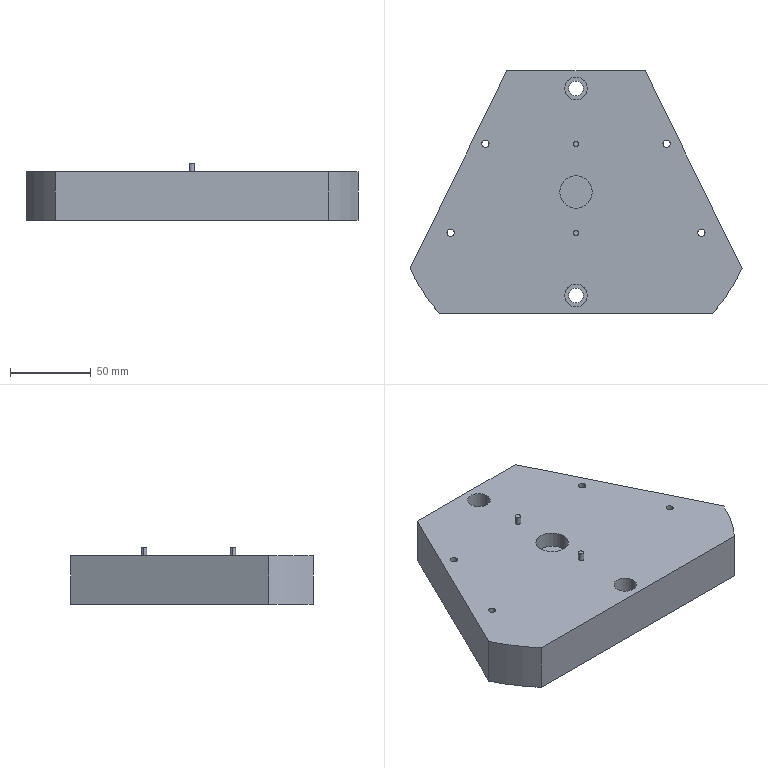Part | 1 solid | 53 faces | volume 676513 mm3 | cylinder 36 | plane 17 | commonest cylinder face diameters 4.5 x8 8 x8 3.3 x4 9 x4 12 x4 14 x4